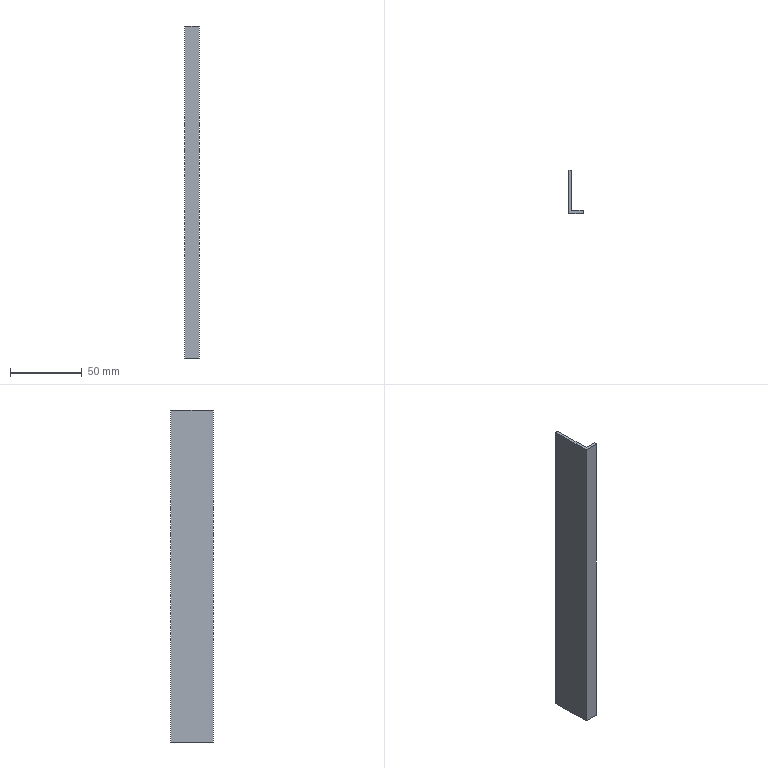Part | SolidWorks | features ExtruThin 1 | 1 solid | 8 faces | box 10 x 30 x 232 mm | volume 17632 mm3 | plane 8
STEP:
#1=CARTESIAN_POINT('',(0.,0.,-116.));
#2=VERTEX_POINT('',#1);
#3=CARTESIAN_POINT('',(10.,0.,-116.));
#4=VERTEX_POINT('',#3);
#5=CARTESIAN_POINT('',(0.,0.,-116.));
#6=DIRECTION('',(1.,0.,0.));
#7=VECTOR('',#6,1000.);
#8=LINE('',#5,#7);
#9=EDGE_CURVE('',#2,#4,#8,.T.);
#10=ORIENTED_EDGE('',*,*,#9,.T.);
#11=CARTESIAN_POINT('',(10.,0.,116.));
#12=VERTEX_POINT('',#11);
#13=CARTESIAN_POINT('',(10.,0.,116.));
#14=DIRECTION('',(0.,0.,-1.));
#15=VECTOR('',#14,1000.);
#16=LINE('',#13,#15);
#17=EDGE_CURVE('',#12,#4,#16,.T.);
#18=ORIENTED_EDGE('',*,*,#17,.F.);
#19=CARTESIAN_POINT('',(0.,0.,116.));
#20=VERTEX_POINT('',#19);
#21=CARTESIAN_POINT('',(0.,0.,116.));
#22=DIRECTION('',(1.,0.,0.));
#23=VECTOR('',#22,1000.);
#24=LINE('',#21,#23);
#25=EDGE_CURVE('',#20,#12,#24,.T.);
#26=ORIENTED_EDGE('',*,*,#25,.F.);
#27=CARTESIAN_POINT('',(0.,0.,116.));
#28=DIRECTION('',(0.,0.,-1.));
#29=VECTOR('',#28,1000.);
#30=LINE('',#27,#29);
#31=EDGE_CURVE('',#20,#2,#30,.T.);
#32=ORIENTED_EDGE('',*,*,#31,.T.);
#33=EDGE_LOOP('',(#10,#18,#26,#32));
#34=FACE_OUTER_BOUND('',#33,.T.);
#35=CARTESIAN_POINT('',(0.,0.,116.));
#36=DIRECTION('',(0.,1.,0.));
#37=DIRECTION('',(0.,0.,1.));
#38=AXIS2_PLACEMENT_3D('',#35,#36,#37);
#39=PLANE('',#38);
#40=ADVANCED_FACE('',(#34),#39,.F.);
#41=CARTESIAN_POINT('',(10.,2.,-116.));
#42=VERTEX_POINT('',#41);
#43=CARTESIAN_POINT('',(10.,2.,-116.));
#44=DIRECTION('',(0.,-1.,0.));
#45=VECTOR('',#44,1000.);
#46=LINE('',#43,#45);
#47=EDGE_CURVE('',#42,#4,#46,.T.);
#48=ORIENTED_EDGE('',*,*,#47,.F.);
#49=CARTESIAN_POINT('',(10.,2.,116.));
#50=VERTEX_POINT('',#49);
#51=CARTESIAN_POINT('',(10.,2.,116.));
#52=DIRECTION('',(0.,0.,-1.));
#53=VECTOR('',#52,1000.);
#54=LINE('',#51,#53);
#55=EDGE_CURVE('',#50,#42,#54,.T.);
#56=ORIENTED_EDGE('',*,*,#55,.F.);
#57=CARTESIAN_POINT('',(10.,2.,116.));
#58=DIRECTION('',(0.,-1.,0.));
#59=VECTOR('',#58,1000.);
#60=LINE('',#57,#59);
#61=EDGE_CURVE('',#50,#12,#60,.T.);
#62=ORIENTED_EDGE('',*,*,#61,.T.);
#63=ORIENTED_EDGE('',*,*,#17,.T.);
#64=EDGE_LOOP('',(#48,#56,#62,#63));
#65=FACE_OUTER_BOUND('',#64,.T.);
#66=CARTESIAN_POINT('',(10.,2.,116.));
#67=DIRECTION('',(1.,0.,0.));
#68=DIRECTION('',(0.,0.,-1.));
#69=AXIS2_PLACEMENT_3D('',#66,#67,#68);
#70=PLANE('',#69);
#71=ADVANCED_FACE('',(#65),#70,.T.);
#72=CARTESIAN_POINT('',(2.,2.,-116.));
#73=VERTEX_POINT('',#72);
#74=CARTESIAN_POINT('',(0.,2.,-116.));
#75=DIRECTION('',(1.,0.,0.));
#76=VECTOR('',#75,1000.);
#77=LINE('',#74,#76);
#78=EDGE_CURVE('',#73,#42,#77,.T.);
#79=ORIENTED_EDGE('',*,*,#78,.F.);
#80=CARTESIAN_POINT('',(2.,2.,116.));
#81=VERTEX_POINT('',#80);
#82=CARTESIAN_POINT('',(2.,2.,116.));
#83=DIRECTION('',(0.,0.,-1.));
#84=VECTOR('',#83,1000.);
#85=LINE('',#82,#84);
#86=EDGE_CURVE('',#81,#73,#85,.T.);
#87=ORIENTED_EDGE('',*,*,#86,.F.);
#88=CARTESIAN_POINT('',(0.,2.,116.));
#89=DIRECTION('',(1.,0.,0.));
#90=VECTOR('',#89,1000.);
#91=LINE('',#88,#90);
#92=EDGE_CURVE('',#81,#50,#91,.T.);
#93=ORIENTED_EDGE('',*,*,#92,.T.);
#94=ORIENTED_EDGE('',*,*,#55,.T.);
#95=EDGE_LOOP('',(#79,#87,#93,#94));
#96=FACE_OUTER_BOUND('',#95,.T.);
#97=CARTESIAN_POINT('',(0.,2.,116.));
#98=DIRECTION('',(0.,1.,0.));
#99=DIRECTION('',(0.,0.,1.));
#100=AXIS2_PLACEMENT_3D('',#97,#98,#99);
#101=PLANE('',#100);
#102=ADVANCED_FACE('',(#96),#101,.T.);
#103=CARTESIAN_POINT('',(2.,30.,-116.));
#104=VERTEX_POINT('',#103);
#105=CARTESIAN_POINT('',(2.,0.,-116.));
#106=DIRECTION('',(0.,-1.,0.));
#107=VECTOR('',#106,1000.);
#108=LINE('',#105,#107);
#109=EDGE_CURVE('',#104,#73,#108,.T.);
#110=ORIENTED_EDGE('',*,*,#109,.F.);
#111=CARTESIAN_POINT('',(2.,30.,116.));
#112=VERTEX_POINT('',#111);
#113=CARTESIAN_POINT('',(2.,30.,116.));
#114=DIRECTION('',(0.,0.,-1.));
#115=VECTOR('',#114,1000.);
#116=LINE('',#113,#115);
#117=EDGE_CURVE('',#112,#104,#116,.T.);
#118=ORIENTED_EDGE('',*,*,#117,.F.);
#119=CARTESIAN_POINT('',(2.,0.,116.));
#120=DIRECTION('',(0.,-1.,0.));
#121=VECTOR('',#120,1000.);
#122=LINE('',#119,#121);
#123=EDGE_CURVE('',#112,#81,#122,.T.);
#124=ORIENTED_EDGE('',*,*,#123,.T.);
#125=ORIENTED_EDGE('',*,*,#86,.T.);
#126=EDGE_LOOP('',(#110,#118,#124,#125));
#127=FACE_OUTER_BOUND('',#126,.T.);
#128=CARTESIAN_POINT('',(2.,0.,116.));
#129=DIRECTION('',(1.,0.,0.));
#130=DIRECTION('',(0.,0.,-1.));
#131=AXIS2_PLACEMENT_3D('',#128,#129,#130);
#132=PLANE('',#131);
#133=ADVANCED_FACE('',(#127),#132,.T.);
#134=CARTESIAN_POINT('',(0.,30.,-116.));
#135=VERTEX_POINT('',#134);
#136=CARTESIAN_POINT('',(0.,30.,-116.));
#137=DIRECTION('',(1.,0.,0.));
#138=VECTOR('',#137,1000.);
#139=LINE('',#136,#138);
#140=EDGE_CURVE('',#135,#104,#139,.T.);
#141=ORIENTED_EDGE('',*,*,#140,.F.);
#142=CARTESIAN_POINT('',(0.,30.,116.));
#143=VERTEX_POINT('',#142);
#144=CARTESIAN_POINT('',(0.,30.,116.));
#145=DIRECTION('',(0.,0.,-1.));
#146=VECTOR('',#145,1000.);
#147=LINE('',#144,#146);
#148=EDGE_CURVE('',#143,#135,#147,.T.);
#149=ORIENTED_EDGE('',*,*,#148,.F.);
#150=CARTESIAN_POINT('',(0.,30.,116.));
#151=DIRECTION('',(1.,0.,0.));
#152=VECTOR('',#151,1000.);
#153=LINE('',#150,#152);
#154=EDGE_CURVE('',#143,#112,#153,.T.);
#155=ORIENTED_EDGE('',*,*,#154,.T.);
#156=ORIENTED_EDGE('',*,*,#117,.T.);
#157=EDGE_LOOP('',(#141,#149,#155,#156));
#158=FACE_OUTER_BOUND('',#157,.T.);
#159=CARTESIAN_POINT('',(0.,30.,116.));
#160=DIRECTION('',(0.,1.,0.));
#161=DIRECTION('',(0.,0.,1.));
#162=AXIS2_PLACEMENT_3D('',#159,#160,#161);
#163=PLANE('',#162);
#164=ADVANCED_FACE('',(#158),#163,.T.);
#165=CARTESIAN_POINT('',(0.,0.,-116.));
#166=DIRECTION('',(0.,-1.,0.));
#167=VECTOR('',#166,1000.);
#168=LINE('',#165,#167);
#169=EDGE_CURVE('',#135,#2,#168,.T.);
#170=ORIENTED_EDGE('',*,*,#169,.T.);
#171=ORIENTED_EDGE('',*,*,#31,.F.);
#172=CARTESIAN_POINT('',(0.,0.,116.));
#173=DIRECTION('',(0.,-1.,0.));
#174=VECTOR('',#173,1000.);
#175=LINE('',#172,#174);
#176=EDGE_CURVE('',#143,#20,#175,.T.);
#177=ORIENTED_EDGE('',*,*,#176,.F.);
#178=ORIENTED_EDGE('',*,*,#148,.T.);
#179=EDGE_LOOP('',(#170,#171,#177,#178));
#180=FACE_OUTER_BOUND('',#179,.T.);
#181=CARTESIAN_POINT('',(0.,0.,116.));
#182=DIRECTION('',(1.,0.,0.));
#183=DIRECTION('',(0.,0.,-1.));
#184=AXIS2_PLACEMENT_3D('',#181,#182,#183);
#185=PLANE('',#184);
#186=ADVANCED_FACE('',(#180),#185,.F.);
#187=ORIENTED_EDGE('',*,*,#25,.T.);
#188=ORIENTED_EDGE('',*,*,#61,.F.);
#189=ORIENTED_EDGE('',*,*,#92,.F.);
#190=ORIENTED_EDGE('',*,*,#123,.F.);
#191=ORIENTED_EDGE('',*,*,#154,.F.);
#192=ORIENTED_EDGE('',*,*,#176,.T.);
#193=EDGE_LOOP('',(#187,#188,#189,#190,#191,#192));
#194=FACE_OUTER_BOUND('',#193,.T.);
#195=CARTESIAN_POINT('',(0.,0.,116.));
#196=DIRECTION('',(0.,0.,-1.));
#197=DIRECTION('',(-1.,0.,0.));
#198=AXIS2_PLACEMENT_3D('',#195,#196,#197);
#199=PLANE('',#198);
#200=ADVANCED_FACE('',(#194),#199,.F.);
#201=ORIENTED_EDGE('',*,*,#9,.F.);
#202=ORIENTED_EDGE('',*,*,#169,.F.);
#203=ORIENTED_EDGE('',*,*,#140,.T.);
#204=ORIENTED_EDGE('',*,*,#109,.T.);
#205=ORIENTED_EDGE('',*,*,#78,.T.);
#206=ORIENTED_EDGE('',*,*,#47,.T.);
#207=EDGE_LOOP('',(#201,#202,#203,#204,#205,#206));
#208=FACE_OUTER_BOUND('',#207,.T.);
#209=CARTESIAN_POINT('',(0.,0.,-116.));
#210=DIRECTION('',(0.,0.,-1.));
#211=DIRECTION('',(-1.,0.,0.));
#212=AXIS2_PLACEMENT_3D('',#209,#210,#211);
#213=PLANE('',#212);
#214=ADVANCED_FACE('',(#208),#213,.T.);
#215=CLOSED_SHELL('',(#40,#71,#102,#133,#164,#186,#200,#214));
#216=MANIFOLD_SOLID_BREP('',#215);
#217=CARTESIAN_POINT('',(0.,0.,0.));
#218=DIRECTION('',(0.,0.,1.));
#219=DIRECTION('',(1.,0.,0.));
#220=AXIS2_PLACEMENT_3D('',#217,#218,#219);
#221=(LENGTH_UNIT()NAMED_UNIT(*)SI_UNIT(.MILLI.,.METRE.));
#222=UNCERTAINTY_MEASURE_WITH_UNIT(LENGTH_MEASURE(0.00001),#221,'','');
#223=(NAMED_UNIT(*)PLANE_ANGLE_UNIT()SI_UNIT($,.RADIAN.));
#224=(NAMED_UNIT(*)SI_UNIT($,.STERADIAN.)SOLID_ANGLE_UNIT());
#225=(GEOMETRIC_REPRESENTATION_CONTEXT(3)GLOBAL_UNCERTAINTY_ASSIGNED_CONTEXT((#222))GLOBAL_UNIT_ASSIGNED_CONTEXT((#221,#223,#224))REPRESENTATION_CONTEXT('',''));
#226=ADVANCED_BREP_SHAPE_REPRESENTATION('',(#216,#220),#225);